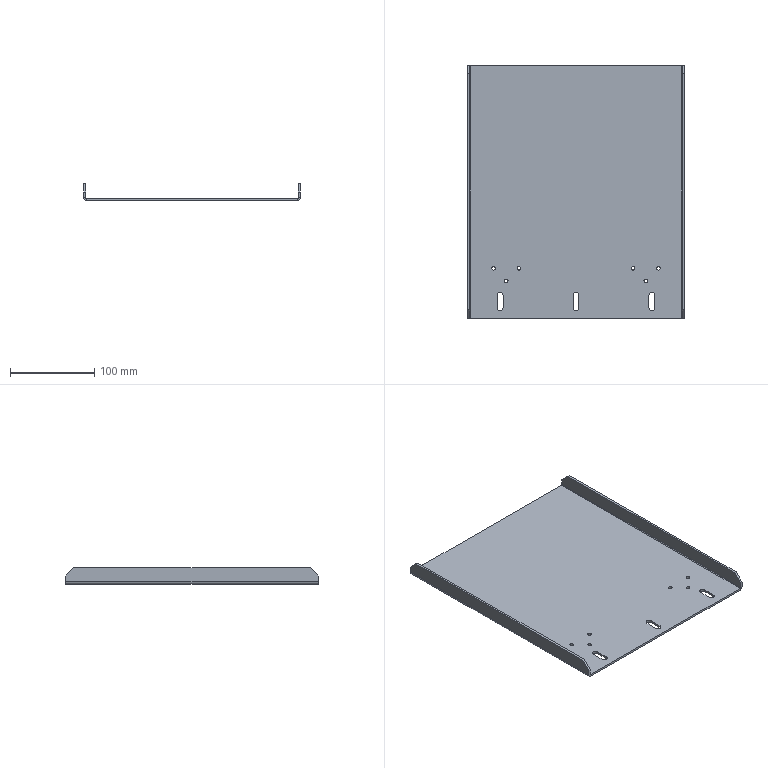Part | SolidWorks | features HoleWzd 2, BreakCorner 1, Chamfer 1, EdgeFlange 1, Extrusion 1, FlatPattern 1, SheetMetal 1, SolidToSheetMetal 1 | 1 solid | 50 faces | box 257 x 300 x 20 mm | volume 215937 mm3 | plane 28 | cylinder 22 | commonest cylinder face diameters 4.2 x12 7 x6 1.473 x2 6.473 x2
STEP:
#1=CARTESIAN_POINT('',(-95.65,-90.5,1.5));
#2=VERTEX_POINT('',#1);
#3=CARTESIAN_POINT('',(-99.85,-90.5,1.5));
#4=VERTEX_POINT('',#3);
#5=CARTESIAN_POINT('',(-97.75,-90.5,1.5));
#6=DIRECTION('',(0.,0.,-1.));
#7=DIRECTION('',(-1.,0.,0.));
#8=AXIS2_PLACEMENT_3D('',#5,#6,#7);
#9=CIRCLE('',#8,2.1);
#10=EDGE_CURVE('',#2,#4,#9,.T.);
#11=ORIENTED_EDGE('',*,*,#10,.F.);
#12=CARTESIAN_POINT('',(-95.65,-90.5,-1.));
#13=VERTEX_POINT('',#12);
#14=CARTESIAN_POINT('',(-95.65,-90.5,1.5));
#15=DIRECTION('',(0.,0.,-1.));
#16=VECTOR('',#15,1000.);
#17=LINE('',#14,#16);
#18=EDGE_CURVE('',#2,#13,#17,.T.);
#19=ORIENTED_EDGE('',*,*,#18,.T.);
#20=CARTESIAN_POINT('',(-99.85,-90.5,-1.));
#21=VERTEX_POINT('',#20);
#22=CARTESIAN_POINT('',(-97.75,-90.5,-1.));
#23=DIRECTION('',(0.,0.,-1.));
#24=DIRECTION('',(-1.,0.,0.));
#25=AXIS2_PLACEMENT_3D('',#22,#23,#24);
#26=CIRCLE('',#25,2.1);
#27=EDGE_CURVE('',#13,#21,#26,.T.);
#28=ORIENTED_EDGE('',*,*,#27,.T.);
#29=CARTESIAN_POINT('',(-99.85,-90.5,1.5));
#30=DIRECTION('',(0.,0.,-1.));
#31=VECTOR('',#30,1000.);
#32=LINE('',#29,#31);
#33=EDGE_CURVE('',#4,#21,#32,.T.);
#34=ORIENTED_EDGE('',*,*,#33,.F.);
#35=EDGE_LOOP('',(#11,#19,#28,#34));
#36=FACE_OUTER_BOUND('',#35,.T.);
#37=CARTESIAN_POINT('',(-97.75,-90.5,1.5));
#38=DIRECTION('',(0.,0.,-1.));
#39=DIRECTION('',(-1.,0.,0.));
#40=AXIS2_PLACEMENT_3D('',#37,#38,#39);
#41=CYLINDRICAL_SURFACE('',#40,2.1);
#42=ADVANCED_FACE('',(#36),#41,.F.);
#43=CARTESIAN_POINT('',(-65.65,-90.5,1.5));
#44=VERTEX_POINT('',#43);
#45=CARTESIAN_POINT('',(-69.85,-90.5,1.5));
#46=VERTEX_POINT('',#45);
#47=CARTESIAN_POINT('',(-67.75,-90.5,1.5));
#48=DIRECTION('',(0.,0.,-1.));
#49=DIRECTION('',(-1.,0.,0.));
#50=AXIS2_PLACEMENT_3D('',#47,#48,#49);
#51=CIRCLE('',#50,2.1);
#52=EDGE_CURVE('',#44,#46,#51,.T.);
#53=ORIENTED_EDGE('',*,*,#52,.F.);
#54=CARTESIAN_POINT('',(-65.65,-90.5,-1.));
#55=VERTEX_POINT('',#54);
#56=CARTESIAN_POINT('',(-65.65,-90.5,1.5));
#57=DIRECTION('',(0.,0.,-1.));
#58=VECTOR('',#57,1000.);
#59=LINE('',#56,#58);
#60=EDGE_CURVE('',#44,#55,#59,.T.);
#61=ORIENTED_EDGE('',*,*,#60,.T.);
#62=CARTESIAN_POINT('',(-69.85,-90.5,-1.));
#63=VERTEX_POINT('',#62);
#64=CARTESIAN_POINT('',(-67.75,-90.5,-1.));
#65=DIRECTION('',(0.,0.,-1.));
#66=DIRECTION('',(-1.,0.,0.));
#67=AXIS2_PLACEMENT_3D('',#64,#65,#66);
#68=CIRCLE('',#67,2.1);
#69=EDGE_CURVE('',#55,#63,#68,.T.);
#70=ORIENTED_EDGE('',*,*,#69,.T.);
#71=CARTESIAN_POINT('',(-69.85,-90.5,1.5));
#72=DIRECTION('',(0.,0.,-1.));
#73=VECTOR('',#72,1000.);
#74=LINE('',#71,#73);
#75=EDGE_CURVE('',#46,#63,#74,.T.);
#76=ORIENTED_EDGE('',*,*,#75,.F.);
#77=EDGE_LOOP('',(#53,#61,#70,#76));
#78=FACE_OUTER_BOUND('',#77,.T.);
#79=CARTESIAN_POINT('',(-67.75,-90.5,1.5));
#80=DIRECTION('',(0.,0.,-1.));
#81=DIRECTION('',(-1.,0.,0.));
#82=AXIS2_PLACEMENT_3D('',#79,#80,#81);
#83=CYLINDRICAL_SURFACE('',#82,2.1);
#84=ADVANCED_FACE('',(#78),#83,.F.);
#85=CARTESIAN_POINT('',(-80.65,-105.5,1.5));
#86=VERTEX_POINT('',#85);
#87=CARTESIAN_POINT('',(-84.85,-105.5,1.5));
#88=VERTEX_POINT('',#87);
#89=CARTESIAN_POINT('',(-82.75,-105.5,1.5));
#90=DIRECTION('',(0.,0.,-1.));
#91=DIRECTION('',(-1.,0.,0.));
#92=AXIS2_PLACEMENT_3D('',#89,#90,#91);
#93=CIRCLE('',#92,2.1);
#94=EDGE_CURVE('',#86,#88,#93,.T.);
#95=ORIENTED_EDGE('',*,*,#94,.F.);
#96=CARTESIAN_POINT('',(-80.65,-105.5,-1.));
#97=VERTEX_POINT('',#96);
#98=CARTESIAN_POINT('',(-80.65,-105.5,1.5));
#99=DIRECTION('',(0.,0.,-1.));
#100=VECTOR('',#99,1000.);
#101=LINE('',#98,#100);
#102=EDGE_CURVE('',#86,#97,#101,.T.);
#103=ORIENTED_EDGE('',*,*,#102,.T.);
#104=CARTESIAN_POINT('',(-84.85,-105.5,-1.));
#105=VERTEX_POINT('',#104);
#106=CARTESIAN_POINT('',(-82.75,-105.5,-1.));
#107=DIRECTION('',(0.,0.,-1.));
#108=DIRECTION('',(-1.,0.,0.));
#109=AXIS2_PLACEMENT_3D('',#106,#107,#108);
#110=CIRCLE('',#109,2.1);
#111=EDGE_CURVE('',#97,#105,#110,.T.);
#112=ORIENTED_EDGE('',*,*,#111,.T.);
#113=CARTESIAN_POINT('',(-84.85,-105.5,1.5));
#114=DIRECTION('',(0.,0.,-1.));
#115=VECTOR('',#114,1000.);
#116=LINE('',#113,#115);
#117=EDGE_CURVE('',#88,#105,#116,.T.);
#118=ORIENTED_EDGE('',*,*,#117,.F.);
#119=EDGE_LOOP('',(#95,#103,#112,#118));
#120=FACE_OUTER_BOUND('',#119,.T.);
#121=CARTESIAN_POINT('',(-82.75,-105.5,1.5));
#122=DIRECTION('',(0.,0.,-1.));
#123=DIRECTION('',(-1.,0.,0.));
#124=AXIS2_PLACEMENT_3D('',#121,#122,#123);
#125=CYLINDRICAL_SURFACE('',#124,2.1);
#126=ADVANCED_FACE('',(#120),#125,.F.);
#127=CARTESIAN_POINT('',(84.85,-105.5,1.5));
#128=VERTEX_POINT('',#127);
#129=CARTESIAN_POINT('',(80.65,-105.5,1.5));
#130=VERTEX_POINT('',#129);
#131=CARTESIAN_POINT('',(82.75,-105.5,1.5));
#132=DIRECTION('',(0.,0.,-1.));
#133=DIRECTION('',(-1.,0.,0.));
#134=AXIS2_PLACEMENT_3D('',#131,#132,#133);
#135=CIRCLE('',#134,2.1);
#136=EDGE_CURVE('',#128,#130,#135,.T.);
#137=ORIENTED_EDGE('',*,*,#136,.F.);
#138=CARTESIAN_POINT('',(84.85,-105.5,-1.));
#139=VERTEX_POINT('',#138);
#140=CARTESIAN_POINT('',(84.85,-105.5,1.5));
#141=DIRECTION('',(0.,0.,-1.));
#142=VECTOR('',#141,1000.);
#143=LINE('',#140,#142);
#144=EDGE_CURVE('',#128,#139,#143,.T.);
#145=ORIENTED_EDGE('',*,*,#144,.T.);
#146=CARTESIAN_POINT('',(80.65,-105.5,-1.));
#147=VERTEX_POINT('',#146);
#148=CARTESIAN_POINT('',(82.75,-105.5,-1.));
#149=DIRECTION('',(0.,0.,-1.));
#150=DIRECTION('',(-1.,0.,0.));
#151=AXIS2_PLACEMENT_3D('',#148,#149,#150);
#152=CIRCLE('',#151,2.1);
#153=EDGE_CURVE('',#139,#147,#152,.T.);
#154=ORIENTED_EDGE('',*,*,#153,.T.);
#155=CARTESIAN_POINT('',(80.65,-105.5,1.5));
#156=DIRECTION('',(0.,0.,-1.));
#157=VECTOR('',#156,1000.);
#158=LINE('',#155,#157);
#159=EDGE_CURVE('',#130,#147,#158,.T.);
#160=ORIENTED_EDGE('',*,*,#159,.F.);
#161=EDGE_LOOP('',(#137,#145,#154,#160));
#162=FACE_OUTER_BOUND('',#161,.T.);
#163=CARTESIAN_POINT('',(82.75,-105.5,1.5));
#164=DIRECTION('',(0.,0.,-1.));
#165=DIRECTION('',(-1.,0.,0.));
#166=AXIS2_PLACEMENT_3D('',#163,#164,#165);
#167=CYLINDRICAL_SURFACE('',#166,2.1);
#168=ADVANCED_FACE('',(#162),#167,.F.);
#169=CARTESIAN_POINT('',(69.85,-90.5,1.5));
#170=VERTEX_POINT('',#169);
#171=CARTESIAN_POINT('',(65.65,-90.5,1.5));
#172=VERTEX_POINT('',#171);
#173=CARTESIAN_POINT('',(67.75,-90.5,1.5));
#174=DIRECTION('',(0.,0.,-1.));
#175=DIRECTION('',(-1.,0.,0.));
#176=AXIS2_PLACEMENT_3D('',#173,#174,#175);
#177=CIRCLE('',#176,2.1);
#178=EDGE_CURVE('',#170,#172,#177,.T.);
#179=ORIENTED_EDGE('',*,*,#178,.F.);
#180=CARTESIAN_POINT('',(69.85,-90.5,-1.));
#181=VERTEX_POINT('',#180);
#182=CARTESIAN_POINT('',(69.85,-90.5,1.5));
#183=DIRECTION('',(0.,0.,-1.));
#184=VECTOR('',#183,1000.);
#185=LINE('',#182,#184);
#186=EDGE_CURVE('',#170,#181,#185,.T.);
#187=ORIENTED_EDGE('',*,*,#186,.T.);
#188=CARTESIAN_POINT('',(65.65,-90.5,-1.));
#189=VERTEX_POINT('',#188);
#190=CARTESIAN_POINT('',(67.75,-90.5,-1.));
#191=DIRECTION('',(0.,0.,-1.));
#192=DIRECTION('',(-1.,0.,0.));
#193=AXIS2_PLACEMENT_3D('',#190,#191,#192);
#194=CIRCLE('',#193,2.1);
#195=EDGE_CURVE('',#181,#189,#194,.T.);
#196=ORIENTED_EDGE('',*,*,#195,.T.);
#197=CARTESIAN_POINT('',(65.65,-90.5,1.5));
#198=DIRECTION('',(0.,0.,-1.));
#199=VECTOR('',#198,1000.);
#200=LINE('',#197,#199);
#201=EDGE_CURVE('',#172,#189,#200,.T.);
#202=ORIENTED_EDGE('',*,*,#201,.F.);
#203=EDGE_LOOP('',(#179,#187,#196,#202));
#204=FACE_OUTER_BOUND('',#203,.T.);
#205=CARTESIAN_POINT('',(67.75,-90.5,1.5));
#206=DIRECTION('',(0.,0.,-1.));
#207=DIRECTION('',(-1.,0.,0.));
#208=AXIS2_PLACEMENT_3D('',#205,#206,#207);
#209=CYLINDRICAL_SURFACE('',#208,2.1);
#210=ADVANCED_FACE('',(#204),#209,.F.);
#211=CARTESIAN_POINT('',(99.85,-90.5,1.5));
#212=VERTEX_POINT('',#211);
#213=CARTESIAN_POINT('',(95.65,-90.5,1.5));
#214=VERTEX_POINT('',#213);
#215=CARTESIAN_POINT('',(97.75,-90.5,1.5));
#216=DIRECTION('',(0.,0.,-1.));
#217=DIRECTION('',(-1.,0.,0.));
#218=AXIS2_PLACEMENT_3D('',#215,#216,#217);
#219=CIRCLE('',#218,2.1);
#220=EDGE_CURVE('',#212,#214,#219,.T.);
#221=ORIENTED_EDGE('',*,*,#220,.F.);
#222=CARTESIAN_POINT('',(99.85,-90.5,-1.));
#223=VERTEX_POINT('',#222);
#224=CARTESIAN_POINT('',(99.85,-90.5,1.5));
#225=DIRECTION('',(0.,0.,-1.));
#226=VECTOR('',#225,1000.);
#227=LINE('',#224,#226);
#228=EDGE_CURVE('',#212,#223,#227,.T.);
#229=ORIENTED_EDGE('',*,*,#228,.T.);
#230=CARTESIAN_POINT('',(95.65,-90.5,-1.));
#231=VERTEX_POINT('',#230);
#232=CARTESIAN_POINT('',(97.75,-90.5,-1.));
#233=DIRECTION('',(0.,0.,-1.));
#234=DIRECTION('',(-1.,0.,0.));
#235=AXIS2_PLACEMENT_3D('',#232,#233,#234);
#236=CIRCLE('',#235,2.1);
#237=EDGE_CURVE('',#223,#231,#236,.T.);
#238=ORIENTED_EDGE('',*,*,#237,.T.);
#239=CARTESIAN_POINT('',(95.65,-90.5,1.5));
#240=DIRECTION('',(0.,0.,-1.));
#241=VECTOR('',#240,1000.);
#242=LINE('',#239,#241);
#243=EDGE_CURVE('',#214,#231,#242,.T.);
#244=ORIENTED_EDGE('',*,*,#243,.F.);
#245=EDGE_LOOP('',(#221,#229,#238,#244));
#246=FACE_OUTER_BOUND('',#245,.T.);
#247=CARTESIAN_POINT('',(97.75,-90.5,1.5));
#248=DIRECTION('',(0.,0.,-1.));
#249=DIRECTION('',(-1.,0.,0.));
#250=AXIS2_PLACEMENT_3D('',#247,#248,#249);
#251=CYLINDRICAL_SURFACE('',#250,2.1);
#252=ADVANCED_FACE('',(#246),#251,.F.);
#253=CARTESIAN_POINT('',(97.75,-90.5,1.5));
#254=DIRECTION('',(0.,0.,-1.));
#255=DIRECTION('',(-1.,0.,0.));
#256=AXIS2_PLACEMENT_3D('',#253,#254,#255);
#257=CIRCLE('',#256,2.1);
#258=EDGE_CURVE('',#214,#212,#257,.T.);
#259=ORIENTED_EDGE('',*,*,#258,.T.);
#260=ORIENTED_EDGE('',*,*,#220,.T.);
#261=EDGE_LOOP('',(#259,#260));
#262=FACE_BOUND('',#261,.T.);
#263=CARTESIAN_POINT('',(67.75,-90.5,1.5));
#264=DIRECTION('',(0.,0.,-1.));
#265=DIRECTION('',(-1.,0.,0.));
#266=AXIS2_PLACEMENT_3D('',#263,#264,#265);
#267=CIRCLE('',#266,2.1);
#268=EDGE_CURVE('',#172,#170,#267,.T.);
#269=ORIENTED_EDGE('',*,*,#268,.T.);
#270=ORIENTED_EDGE('',*,*,#178,.T.);
#271=EDGE_LOOP('',(#269,#270));
#272=FACE_BOUND('',#271,.T.);
#273=CARTESIAN_POINT('',(82.75,-105.5,1.5));
#274=DIRECTION('',(0.,0.,-1.));
#275=DIRECTION('',(-1.,0.,0.));
#276=AXIS2_PLACEMENT_3D('',#273,#274,#275);
#277=CIRCLE('',#276,2.1);
#278=EDGE_CURVE('',#130,#128,#277,.T.);
#279=ORIENTED_EDGE('',*,*,#278,.T.);
#280=ORIENTED_EDGE('',*,*,#136,.T.);
#281=EDGE_LOOP('',(#279,#280));
#282=FACE_BOUND('',#281,.T.);
#283=CARTESIAN_POINT('',(-82.75,-105.5,1.5));
#284=DIRECTION('',(0.,0.,-1.));
#285=DIRECTION('',(-1.,0.,0.));
#286=AXIS2_PLACEMENT_3D('',#283,#284,#285);
#287=CIRCLE('',#286,2.1);
#288=EDGE_CURVE('',#88,#86,#287,.T.);
#289=ORIENTED_EDGE('',*,*,#288,.T.);
#290=ORIENTED_EDGE('',*,*,#94,.T.);
#291=EDGE_LOOP('',(#289,#290));
#292=FACE_BOUND('',#291,.T.);
#293=CARTESIAN_POINT('',(-67.75,-90.5,1.5));
#294=DIRECTION('',(0.,0.,-1.));
#295=DIRECTION('',(-1.,0.,0.));
#296=AXIS2_PLACEMENT_3D('',#293,#294,#295);
#297=CIRCLE('',#296,2.1);
#298=EDGE_CURVE('',#46,#44,#297,.T.);
#299=ORIENTED_EDGE('',*,*,#298,.T.);
#300=ORIENTED_EDGE('',*,*,#52,.T.);
#301=EDGE_LOOP('',(#299,#300));
#302=FACE_BOUND('',#301,.T.);
#303=CARTESIAN_POINT('',(-97.75,-90.5,1.5));
#304=DIRECTION('',(0.,0.,-1.));
#305=DIRECTION('',(-1.,0.,0.));
#306=AXIS2_PLACEMENT_3D('',#303,#304,#305);
#307=CIRCLE('',#306,2.1);
#308=EDGE_CURVE('',#4,#2,#307,.T.);
#309=ORIENTED_EDGE('',*,*,#308,.T.);
#310=ORIENTED_EDGE('',*,*,#10,.T.);
#311=EDGE_LOOP('',(#309,#310));
#312=FACE_BOUND('',#311,.T.);
#313=CARTESIAN_POINT('',(93.5,-137.5,1.5));
#314=VERTEX_POINT('',#313);
#315=CARTESIAN_POINT('',(93.5,-122.5,1.5));
#316=VERTEX_POINT('',#315);
#317=CARTESIAN_POINT('',(93.5,-137.5,1.5));
#318=DIRECTION('',(0.,1.,0.));
#319=VECTOR('',#318,1000.);
#320=LINE('',#317,#319);
#321=EDGE_CURVE('',#314,#316,#320,.T.);
#322=ORIENTED_EDGE('',*,*,#321,.F.);
#323=CARTESIAN_POINT('',(86.5,-137.5,1.5));
#324=VERTEX_POINT('',#323);
#325=CARTESIAN_POINT('',(90.,-137.5,1.5));
#326=DIRECTION('',(0.,0.,-1.));
#327=DIRECTION('',(-1.,0.,0.));
#328=AXIS2_PLACEMENT_3D('',#325,#326,#327);
#329=CIRCLE('',#328,3.5);
#330=EDGE_CURVE('',#314,#324,#329,.T.);
#331=ORIENTED_EDGE('',*,*,#330,.T.);
#332=CARTESIAN_POINT('',(86.5,-122.5,1.5));
#333=VERTEX_POINT('',#332);
#334=CARTESIAN_POINT('',(86.5,-137.5,1.5));
#335=DIRECTION('',(0.,1.,0.));
#336=VECTOR('',#335,1000.);
#337=LINE('',#334,#336);
#338=EDGE_CURVE('',#324,#333,#337,.T.);
#339=ORIENTED_EDGE('',*,*,#338,.T.);
#340=CARTESIAN_POINT('',(90.,-122.5,1.5));
#341=DIRECTION('',(0.,0.,-1.));
#342=DIRECTION('',(-1.,0.,0.));
#343=AXIS2_PLACEMENT_3D('',#340,#341,#342);
#344=CIRCLE('',#343,3.5);
#345=EDGE_CURVE('',#333,#316,#344,.T.);
#346=ORIENTED_EDGE('',*,*,#345,.T.);
#347=EDGE_LOOP('',(#322,#331,#339,#346));
#348=FACE_BOUND('',#347,.T.);
#349=CARTESIAN_POINT('',(-93.5,-137.5,1.5));
#350=VERTEX_POINT('',#349);
#351=CARTESIAN_POINT('',(-93.5,-122.5,1.5));
#352=VERTEX_POINT('',#351);
#353=CARTESIAN_POINT('',(-93.5,-137.5,1.5));
#354=DIRECTION('',(0.,1.,0.));
#355=VECTOR('',#354,1000.);
#356=LINE('',#353,#355);
#357=EDGE_CURVE('',#350,#352,#356,.T.);
#358=ORIENTED_EDGE('',*,*,#357,.T.);
#359=CARTESIAN_POINT('',(-86.5,-122.5,1.5));
#360=VERTEX_POINT('',#359);
#361=CARTESIAN_POINT('',(-90.,-122.5,1.5));
#362=DIRECTION('',(0.,0.,-1.));
#363=DIRECTION('',(-1.,0.,0.));
#364=AXIS2_PLACEMENT_3D('',#361,#362,#363);
#365=CIRCLE('',#364,3.5);
#366=EDGE_CURVE('',#352,#360,#365,.T.);
#367=ORIENTED_EDGE('',*,*,#366,.T.);
#368=CARTESIAN_POINT('',(-86.5,-137.5,1.5));
#369=VERTEX_POINT('',#368);
#370=CARTESIAN_POINT('',(-86.5,-137.5,1.5));
#371=DIRECTION('',(0.,1.,0.));
#372=VECTOR('',#371,1000.);
#373=LINE('',#370,#372);
#374=EDGE_CURVE('',#369,#360,#373,.T.);
#375=ORIENTED_EDGE('',*,*,#374,.F.);
#376=CARTESIAN_POINT('',(-90.,-137.5,1.5));
#377=DIRECTION('',(0.,0.,-1.));
#378=DIRECTION('',(-1.,0.,0.));
#379=AXIS2_PLACEMENT_3D('',#376,#377,#378);
#380=CIRCLE('',#379,3.5);
#381=EDGE_CURVE('',#369,#350,#380,.T.);
#382=ORIENTED_EDGE('',*,*,#381,.T.);
#383=EDGE_LOOP('',(#358,#367,#375,#382));
#384=FACE_BOUND('',#383,.T.);
#385=CARTESIAN_POINT('',(3.5,-137.5,1.5));
#386=VERTEX_POINT('',#385);
#387=CARTESIAN_POINT('',(3.5,-122.5,1.5));
#388=VERTEX_POINT('',#387);
#389=CARTESIAN_POINT('',(3.5,-137.5,1.5));
#390=DIRECTION('',(0.,1.,0.));
#391=VECTOR('',#390,1000.);
#392=LINE('',#389,#391);
#393=EDGE_CURVE('',#386,#388,#392,.T.);
#394=ORIENTED_EDGE('',*,*,#393,.F.);
#395=CARTESIAN_POINT('',(-3.5,-137.5,1.5));
#396=VERTEX_POINT('',#395);
#397=CARTESIAN_POINT('',(0.,-137.5,1.5));
#398=DIRECTION('',(0.,0.,-1.));
#399=DIRECTION('',(-1.,0.,0.));
#400=AXIS2_PLACEMENT_3D('',#397,#398,#399);
#401=CIRCLE('',#400,3.5);
#402=EDGE_CURVE('',#386,#396,#401,.T.);
#403=ORIENTED_EDGE('',*,*,#402,.T.);
#404=CARTESIAN_POINT('',(-3.5,-122.5,1.5));
#405=VERTEX_POINT('',#404);
#406=CARTESIAN_POINT('',(-3.5,-137.5,1.5));
#407=DIRECTION('',(0.,1.,0.));
#408=VECTOR('',#407,1000.);
#409=LINE('',#406,#408);
#410=EDGE_CURVE('',#396,#405,#409,.T.);
#411=ORIENTED_EDGE('',*,*,#410,.T.);
#412=CARTESIAN_POINT('',(0.,-122.5,1.5));
#413=DIRECTION('',(0.,0.,-1.));
#414=DIRECTION('',(-1.,0.,0.));
#415=AXIS2_PLACEMENT_3D('',#412,#413,#414);
#416=CIRCLE('',#415,3.5);
#417=EDGE_CURVE('',#405,#388,#416,.T.);
#418=ORIENTED_EDGE('',*,*,#417,.T.);
#419=EDGE_LOOP('',(#394,#403,#411,#418));
#420=FACE_BOUND('',#419,.T.);
#421=CARTESIAN_POINT('',(-125.263,-150.,1.5));
#422=VERTEX_POINT('',#421);
#423=CARTESIAN_POINT('',(-125.263,150.,1.5));
#424=VERTEX_POINT('',#423);
#425=CARTESIAN_POINT('',(-125.263,-150.,1.5));
#426=DIRECTION('',(0.,1.,0.));
#427=VECTOR('',#426,1000.);
#428=LINE('',#425,#427);
#429=EDGE_CURVE('',#422,#424,#428,.T.);
#430=ORIENTED_EDGE('',*,*,#429,.F.);
#431=CARTESIAN_POINT('',(125.263,-150.,1.5));
#432=VERTEX_POINT('',#431);
#433=CARTESIAN_POINT('',(-126.,-150.,1.5));
#434=DIRECTION('',(1.,0.,0.));
#435=VECTOR('',#434,1000.);
#436=LINE('',#433,#435);
#437=EDGE_CURVE('',#422,#432,#436,.T.);
#438=ORIENTED_EDGE('',*,*,#437,.T.);
#439=CARTESIAN_POINT('',(125.263,150.,1.5));
#440=VERTEX_POINT('',#439);
#441=CARTESIAN_POINT('',(125.263,150.,1.5));
#442=DIRECTION('',(0.,-1.,0.));
#443=VECTOR('',#442,1000.);
#444=LINE('',#441,#443);
#445=EDGE_CURVE('',#440,#432,#444,.T.);
#446=ORIENTED_EDGE('',*,*,#445,.F.);
#447=CARTESIAN_POINT('',(-126.,150.,1.5));
#448=DIRECTION('',(-1.,0.,0.));
#449=VECTOR('',#448,1000.);
#450=LINE('',#447,#449);
#451=EDGE_CURVE('',#440,#424,#450,.T.);
#452=ORIENTED_EDGE('',*,*,#451,.T.);
#453=EDGE_LOOP('',(#430,#438,#446,#452));
#454=FACE_OUTER_BOUND('',#453,.T.);
#455=CARTESIAN_POINT('',(0.,0.,1.5));
#456=DIRECTION('',(0.,0.,-1.));
#457=DIRECTION('',(-1.,0.,0.));
#458=AXIS2_PLACEMENT_3D('',#455,#456,#457);
#459=PLANE('',#458);
#460=ADVANCED_FACE('',(#262,#272,#282,#292,#302,#312,#348,#384,#420,#454),#459,.F.);
#461=CARTESIAN_POINT('',(97.75,-90.5,-1.));
#462=DIRECTION('',(0.,0.,-1.));
#463=DIRECTION('',(-1.,0.,0.));
#464=AXIS2_PLACEMENT_3D('',#461,#462,#463);
#465=CIRCLE('',#464,2.1);
#466=EDGE_CURVE('',#231,#223,#465,.T.);
#467=ORIENTED_EDGE('',*,*,#466,.F.);
#468=ORIENTED_EDGE('',*,*,#237,.F.);
#469=EDGE_LOOP('',(#467,#468));
#470=FACE_BOUND('',#469,.T.);
#471=CARTESIAN_POINT('',(67.75,-90.5,-1.));
#472=DIRECTION('',(0.,0.,-1.));
#473=DIRECTION('',(-1.,0.,0.));
#474=AXIS2_PLACEMENT_3D('',#471,#472,#473);
#475=CIRCLE('',#474,2.1);
#476=EDGE_CURVE('',#189,#181,#475,.T.);
#477=ORIENTED_EDGE('',*,*,#476,.F.);
#478=ORIENTED_EDGE('',*,*,#195,.F.);
#479=EDGE_LOOP('',(#477,#478));
#480=FACE_BOUND('',#479,.T.);
#481=CARTESIAN_POINT('',(82.75,-105.5,-1.));
#482=DIRECTION('',(0.,0.,-1.));
#483=DIRECTION('',(-1.,0.,0.));
#484=AXIS2_PLACEMENT_3D('',#481,#482,#483);
#485=CIRCLE('',#484,2.1);
#486=EDGE_CURVE('',#147,#139,#485,.T.);
#487=ORIENTED_EDGE('',*,*,#486,.F.);
#488=ORIENTED_EDGE('',*,*,#153,.F.);
#489=EDGE_LOOP('',(#487,#488));
#490=FACE_BOUND('',#489,.T.);
#491=CARTESIAN_POINT('',(-82.75,-105.5,-1.));
#492=DIRECTION('',(0.,0.,-1.));
#493=DIRECTION('',(-1.,0.,0.));
#494=AXIS2_PLACEMENT_3D('',#491,#492,#493);
#495=CIRCLE('',#494,2.1);
#496=EDGE_CURVE('',#105,#97,#495,.T.);
#497=ORIENTED_EDGE('',*,*,#496,.F.);
#498=ORIENTED_EDGE('',*,*,#111,.F.);
#499=EDGE_LOOP('',(#497,#498));
#500=FACE_BOUND('',#499,.T.);
#501=CARTESIAN_POINT('',(-67.75,-90.5,-1.));
#502=DIRECTION('',(0.,0.,-1.));
#503=DIRECTION('',(-1.,0.,0.));
#504=AXIS2_PLACEMENT_3D('',#501,#502,#503);
#505=CIRCLE('',#504,2.1);
#506=EDGE_CURVE('',#63,#55,#505,.T.);
#507=ORIENTED_EDGE('',*,*,#506,.F.);
#508=ORIENTED_EDGE('',*,*,#69,.F.);
#509=EDGE_LOOP('',(#507,#508));
#510=FACE_BOUND('',#509,.T.);
#511=CARTESIAN_POINT('',(-97.75,-90.5,-1.));
#512=DIRECTION('',(0.,0.,-1.));
#513=DIRECTION('',(-1.,0.,0.));
#514=AXIS2_PLACEMENT_3D('',#511,#512,#513);
#515=CIRCLE('',#514,2.1);
#516=EDGE_CURVE('',#21,#13,#515,.T.);
#517=ORIENTED_EDGE('',*,*,#516,.F.);
#518=ORIENTED_EDGE('',*,*,#27,.F.);
#519=EDGE_LOOP('',(#517,#518));
#520=FACE_BOUND('',#519,.T.);
#521=CARTESIAN_POINT('',(93.5,-137.5,-1.));
#522=VERTEX_POINT('',#521);
#523=CARTESIAN_POINT('',(93.5,-122.5,-1.));
#524=VERTEX_POINT('',#523);
#525=CARTESIAN_POINT('',(93.5,0.,-1.));
#526=DIRECTION('',(0.,1.,0.));
#527=VECTOR('',#526,1000.);
#528=LINE('',#525,#527);
#529=EDGE_CURVE('',#522,#524,#528,.T.);
#530=ORIENTED_EDGE('',*,*,#529,.T.);
#531=CARTESIAN_POINT('',(86.5,-122.5,-1.));
#532=VERTEX_POINT('',#531);
#533=CARTESIAN_POINT('',(90.,-122.5,-1.));
#534=DIRECTION('',(0.,0.,-1.));
#535=DIRECTION('',(-1.,0.,0.));
#536=AXIS2_PLACEMENT_3D('',#533,#534,#535);
#537=CIRCLE('',#536,3.5);
#538=EDGE_CURVE('',#532,#524,#537,.T.);
#539=ORIENTED_EDGE('',*,*,#538,.F.);
#540=CARTESIAN_POINT('',(86.5,-137.5,-1.));
#541=VERTEX_POINT('',#540);
#542=CARTESIAN_POINT('',(86.5,0.,-1.));
#543=DIRECTION('',(0.,1.,0.));
#544=VECTOR('',#543,1000.);
#545=LINE('',#542,#544);
#546=EDGE_CURVE('',#541,#532,#545,.T.);
#547=ORIENTED_EDGE('',*,*,#546,.F.);
#548=CARTESIAN_POINT('',(90.,-137.5,-1.));
#549=DIRECTION('',(0.,0.,-1.));
#550=DIRECTION('',(-1.,0.,0.));
#551=AXIS2_PLACEMENT_3D('',#548,#549,#550);
#552=CIRCLE('',#551,3.5);
#553=EDGE_CURVE('',#522,#541,#552,.T.);
#554=ORIENTED_EDGE('',*,*,#553,.F.);
#555=EDGE_LOOP('',(#530,#539,#547,#554));
#556=FACE_BOUND('',#555,.T.);
#557=CARTESIAN_POINT('',(-93.5,-137.5,-1.));
#558=VERTEX_POINT('',#557);
#559=CARTESIAN_POINT('',(-93.5,-122.5,-1.));
#560=VERTEX_POINT('',#559);
#561=CARTESIAN_POINT('',(-93.5,0.,-1.));
#562=DIRECTION('',(0.,1.,0.));
#563=VECTOR('',#562,1000.);
#564=LINE('',#561,#563);
#565=EDGE_CURVE('',#558,#560,#564,.T.);
#566=ORIENTED_EDGE('',*,*,#565,.F.);
#567=CARTESIAN_POINT('',(-86.5,-137.5,-1.));
#568=VERTEX_POINT('',#567);
#569=CARTESIAN_POINT('',(-90.,-137.5,-1.));
#570=DIRECTION('',(0.,0.,-1.));
#571=DIRECTION('',(-1.,0.,0.));
#572=AXIS2_PLACEMENT_3D('',#569,#570,#571);
#573=CIRCLE('',#572,3.5);
#574=EDGE_CURVE('',#568,#558,#573,.T.);
#575=ORIENTED_EDGE('',*,*,#574,.F.);
#576=CARTESIAN_POINT('',(-86.5,-122.5,-1.));
#577=VERTEX_POINT('',#576);
#578=CARTESIAN_POINT('',(-86.5,0.,-1.));
#579=DIRECTION('',(0.,1.,0.));
#580=VECTOR('',#579,1000.);
#581=LINE('',#578,#580);
#582=EDGE_CURVE('',#568,#577,#581,.T.);
#583=ORIENTED_EDGE('',*,*,#582,.T.);
#584=CARTESIAN_POINT('',(-90.,-122.5,-1.));
#585=DIRECTION('',(0.,0.,-1.));
#586=DIRECTION('',(-1.,0.,0.));
#587=AXIS2_PLACEMENT_3D('',#584,#585,#586);
#588=CIRCLE('',#587,3.5);
#589=EDGE_CURVE('',#560,#577,#588,.T.);
#590=ORIENTED_EDGE('',*,*,#589,.F.);
#591=EDGE_LOOP('',(#566,#575,#583,#590));
#592=FACE_BOUND('',#591,.T.);
#593=CARTESIAN_POINT('',(3.5,-137.5,-1.));
#594=VERTEX_POINT('',#593);
#595=CARTESIAN_POINT('',(3.5,-122.5,-1.));
#596=VERTEX_POINT('',#595);
#597=CARTESIAN_POINT('',(3.5,0.,-1.));
#598=DIRECTION('',(0.,1.,0.));
#599=VECTOR('',#598,1000.);
#600=LINE('',#597,#599);
#601=EDGE_CURVE('',#594,#596,#600,.T.);
#602=ORIENTED_EDGE('',*,*,#601,.T.);
#603=CARTESIAN_POINT('',(-3.5,-122.5,-1.));
#604=VERTEX_POINT('',#603);
#605=CARTESIAN_POINT('',(0.,-122.5,-1.));
#606=DIRECTION('',(0.,0.,-1.));
#607=DIRECTION('',(-1.,0.,0.));
#608=AXIS2_PLACEMENT_3D('',#605,#606,#607);
#609=CIRCLE('',#608,3.5);
#610=EDGE_CURVE('',#604,#596,#609,.T.);
#611=ORIENTED_EDGE('',*,*,#610,.F.);
#612=CARTESIAN_POINT('',(-3.5,-137.5,-1.));
#613=VERTEX_POINT('',#612);
#614=CARTESIAN_POINT('',(-3.5,0.,-1.));
#615=DIRECTION('',(0.,1.,0.));
#616=VECTOR('',#615,1000.);
#617=LINE('',#614,#616);
#618=EDGE_CURVE('',#613,#604,#617,.T.);
#619=ORIENTED_EDGE('',*,*,#618,.F.);
#620=CARTESIAN_POINT('',(0.,-137.5,-1.));
#621=DIRECTION('',(0.,0.,-1.));
#622=DIRECTION('',(-1.,0.,0.));
#623=AXIS2_PLACEMENT_3D('',#620,#621,#622);
#624=CIRCLE('',#623,3.5);
#625=EDGE_CURVE('',#594,#613,#624,.T.);
#626=ORIENTED_EDGE('',*,*,#625,.F.);
#627=EDGE_LOOP('',(#602,#611,#619,#626));
#628=FACE_BOUND('',#627,.T.);
#629=CARTESIAN_POINT('',(-125.263,-150.,-1.));
#630=VERTEX_POINT('',#629);
#631=CARTESIAN_POINT('',(125.263,-150.,-1.));
#632=VERTEX_POINT('',#631);
#633=CARTESIAN_POINT('',(0.,-150.,-1.));
#634=DIRECTION('',(1.,0.,0.));
#635=VECTOR('',#634,1000.);
#636=LINE('',#633,#635);
#637=EDGE_CURVE('',#630,#632,#636,.T.);
#638=ORIENTED_EDGE('',*,*,#637,.F.);
#639=CARTESIAN_POINT('',(-125.263,150.,-1.));
#640=VERTEX_POINT('',#639);
#641=CARTESIAN_POINT('',(-125.263,-150.,-1.));
#642=DIRECTION('',(0.,1.,0.));
#643=VECTOR('',#642,1000.);
#644=LINE('',#641,#643);
#645=EDGE_CURVE('',#630,#640,#644,.T.);
#646=ORIENTED_EDGE('',*,*,#645,.T.);
#647=CARTESIAN_POINT('',(125.263,150.,-1.));
#648=VERTEX_POINT('',#647);
#649=CARTESIAN_POINT('',(0.,150.,-1.));
#650=DIRECTION('',(-1.,0.,0.));
#651=VECTOR('',#650,1000.);
#652=LINE('',#649,#651);
#653=EDGE_CURVE('',#648,#640,#652,.T.);
#654=ORIENTED_EDGE('',*,*,#653,.F.);
#655=CARTESIAN_POINT('',(125.263,150.,-1.));
#656=DIRECTION('',(0.,-1.,0.));
#657=VECTOR('',#656,1000.);
#658=LINE('',#655,#657);
#659=EDGE_CURVE('',#648,#632,#658,.T.);
#660=ORIENTED_EDGE('',*,*,#659,.T.);
#661=EDGE_LOOP('',(#638,#646,#654,#660));
#662=FACE_OUTER_BOUND('',#661,.T.);
#663=CARTESIAN_POINT('',(0.,0.,-1.));
#664=DIRECTION('',(0.,0.,-1.));
#665=DIRECTION('',(-1.,0.,0.));
#666=AXIS2_PLACEMENT_3D('',#663,#664,#665);
#667=PLANE('',#666);
#668=ADVANCED_FACE('',(#470,#480,#490,#500,#510,#520,#556,#592,#628,#662),#667,.T.);
#669=ORIENTED_EDGE('',*,*,#437,.F.);
#670=CARTESIAN_POINT('',(-125.263,-150.,1.5));
#671=DIRECTION('',(0.,0.,-1.));
#672=VECTOR('',#671,1000.);
#673=LINE('',#670,#672);
#674=EDGE_CURVE('',#422,#630,#673,.T.);
#675=ORIENTED_EDGE('',*,*,#674,.T.);
#676=ORIENTED_EDGE('',*,*,#637,.T.);
#677=CARTESIAN_POINT('',(125.263,-150.,1.5));
#678=DIRECTION('',(0.,0.,-1.));
#679=VECTOR('',#678,1000.);
#680=LINE('',#677,#679);
#681=EDGE_CURVE('',#432,#632,#680,.T.);
#682=ORIENTED_EDGE('',*,*,#681,.F.);
#683=EDGE_LOOP('',(#669,#675,#676,#682));
#684=FACE_OUTER_BOUND('',#683,.T.);
#685=CARTESIAN_POINT('',(-126.,-150.,1.5));
#686=DIRECTION('',(0.,1.,0.));
#687=DIRECTION('',(1.,0.,0.));
#688=AXIS2_PLACEMENT_3D('',#685,#686,#687);
#689=PLANE('',#688);
#690=ADVANCED_FACE('',(#684),#689,.F.);
#691=CARTESIAN_POINT('',(-125.263,150.,1.5));
#692=DIRECTION('',(0.,0.,-1.));
#693=VECTOR('',#692,1000.);
#694=LINE('',#691,#693);
#695=EDGE_CURVE('',#424,#640,#694,.T.);
#696=ORIENTED_EDGE('',*,*,#695,.F.);
#697=ORIENTED_EDGE('',*,*,#451,.F.);
#698=CARTESIAN_POINT('',(125.263,150.,1.5));
#699=DIRECTION('',(0.,0.,-1.));
#700=VECTOR('',#699,1000.);
#701=LINE('',#698,#700);
#702=EDGE_CURVE('',#440,#648,#701,.T.);
#703=ORIENTED_EDGE('',*,*,#702,.T.);
#704=ORIENTED_EDGE('',*,*,#653,.T.);
#705=EDGE_LOOP('',(#696,#697,#703,#704));
#706=FACE_OUTER_BOUND('',#705,.T.);
#707=CARTESIAN_POINT('',(-126.,150.,1.5));
#708=DIRECTION('',(0.,-1.,0.));
#709=DIRECTION('',(-1.,0.,0.));
#710=AXIS2_PLACEMENT_3D('',#707,#708,#709);
#711=PLANE('',#710);
#712=ADVANCED_FACE('',(#706),#711,.F.);
#713=CARTESIAN_POINT('',(-3.5,-137.5,1.5));
#714=DIRECTION('',(0.,0.,1.));
#715=VECTOR('',#714,1000.);
#716=LINE('',#713,#715);
#717=EDGE_CURVE('',#613,#396,#716,.T.);
#718=ORIENTED_EDGE('',*,*,#717,.F.);
#719=ORIENTED_EDGE('',*,*,#618,.T.);
#720=CARTESIAN_POINT('',(-3.5,-122.5,1.5));
#721=DIRECTION('',(0.,0.,1.));
#722=VECTOR('',#721,1000.);
#723=LINE('',#720,#722);
#724=EDGE_CURVE('',#604,#405,#723,.T.);
#725=ORIENTED_EDGE('',*,*,#724,.T.);
#726=ORIENTED_EDGE('',*,*,#410,.F.);
#727=EDGE_LOOP('',(#718,#719,#725,#726));
#728=FACE_OUTER_BOUND('',#727,.T.);
#729=CARTESIAN_POINT('',(-3.5,-137.5,1.5));
#730=DIRECTION('',(-1.,0.,0.));
#731=DIRECTION('',(0.,1.,0.));
#732=AXIS2_PLACEMENT_3D('',#729,#730,#731);
#733=PLANE('',#732);
#734=ADVANCED_FACE('',(#728),#733,.F.);
#735=ORIENTED_EDGE('',*,*,#724,.F.);
#736=ORIENTED_EDGE('',*,*,#610,.T.);
#737=CARTESIAN_POINT('',(3.5,-122.5,1.5));
#738=DIRECTION('',(0.,0.,1.));
#739=VECTOR('',#738,1000.);
#740=LINE('',#737,#739);
#741=EDGE_CURVE('',#596,#388,#740,.T.);
#742=ORIENTED_EDGE('',*,*,#741,.T.);
#743=ORIENTED_EDGE('',*,*,#417,.F.);
#744=EDGE_LOOP('',(#735,#736,#742,#743));
#745=FACE_OUTER_BOUND('',#744,.T.);
#746=CARTESIAN_POINT('',(0.,-122.5,1.5));
#747=DIRECTION('',(0.,0.,-1.));
#748=DIRECTION('',(-1.,0.,0.));
#749=AXIS2_PLACEMENT_3D('',#746,#747,#748);
#750=CYLINDRICAL_SURFACE('',#749,3.5);
#751=ADVANCED_FACE('',(#745),#750,.F.);
#752=ORIENTED_EDGE('',*,*,#741,.F.);
#753=ORIENTED_EDGE('',*,*,#601,.F.);
#754=CARTESIAN_POINT('',(3.5,-137.5,1.5));
#755=DIRECTION('',(0.,0.,1.));
#756=VECTOR('',#755,1000.);
#757=LINE('',#754,#756);
#758=EDGE_CURVE('',#594,#386,#757,.T.);
#759=ORIENTED_EDGE('',*,*,#758,.T.);
#760=ORIENTED_EDGE('',*,*,#393,.T.);
#761=EDGE_LOOP('',(#752,#753,#759,#760));
#762=FACE_OUTER_BOUND('',#761,.T.);
#763=CARTESIAN_POINT('',(3.5,-137.5,1.5));
#764=DIRECTION('',(-1.,0.,0.));
#765=DIRECTION('',(0.,1.,0.));
#766=AXIS2_PLACEMENT_3D('',#763,#764,#765);
#767=PLANE('',#766);
#768=ADVANCED_FACE('',(#762),#767,.T.);
#769=CARTESIAN_POINT('',(-86.5,-122.5,1.5));
#770=DIRECTION('',(0.,0.,1.));
#771=VECTOR('',#770,1000.);
#772=LINE('',#769,#771);
#773=EDGE_CURVE('',#577,#360,#772,.T.);
#774=ORIENTED_EDGE('',*,*,#773,.F.);
#775=ORIENTED_EDGE('',*,*,#582,.F.);
#776=CARTESIAN_POINT('',(-86.5,-137.5,1.5));
#777=DIRECTION('',(0.,0.,1.));
#778=VECTOR('',#777,1000.);
#779=LINE('',#776,#778);
#780=EDGE_CURVE('',#568,#369,#779,.T.);
#781=ORIENTED_EDGE('',*,*,#780,.T.);
#782=ORIENTED_EDGE('',*,*,#374,.T.);
#783=EDGE_LOOP('',(#774,#775,#781,#782));
#784=FACE_OUTER_BOUND('',#783,.T.);
#785=CARTESIAN_POINT('',(-86.5,-137.5,1.5));
#786=DIRECTION('',(-1.,0.,0.));
#787=DIRECTION('',(0.,1.,0.));
#788=AXIS2_PLACEMENT_3D('',#785,#786,#787);
#789=PLANE('',#788);
#790=ADVANCED_FACE('',(#784),#789,.T.);
#791=ORIENTED_EDGE('',*,*,#780,.F.);
#792=ORIENTED_EDGE('',*,*,#574,.T.);
#793=CARTESIAN_POINT('',(-93.5,-137.5,1.5));
#794=DIRECTION('',(0.,0.,1.));
#795=VECTOR('',#794,1000.);
#796=LINE('',#793,#795);
#797=EDGE_CURVE('',#558,#350,#796,.T.);
#798=ORIENTED_EDGE('',*,*,#797,.T.);
#799=ORIENTED_EDGE('',*,*,#381,.F.);
#800=EDGE_LOOP('',(#791,#792,#798,#799));
#801=FACE_OUTER_BOUND('',#800,.T.);
#802=CARTESIAN_POINT('',(-90.,-137.5,1.5));
#803=DIRECTION('',(0.,0.,-1.));
#804=DIRECTION('',(-1.,0.,0.));
#805=AXIS2_PLACEMENT_3D('',#802,#803,#804);
#806=CYLINDRICAL_SURFACE('',#805,3.5);
#807=ADVANCED_FACE('',(#801),#806,.F.);
#808=ORIENTED_EDGE('',*,*,#797,.F.);
#809=ORIENTED_EDGE('',*,*,#565,.T.);
#810=CARTESIAN_POINT('',(-93.5,-122.5,1.5));
#811=DIRECTION('',(0.,0.,1.));
#812=VECTOR('',#811,1000.);
#813=LINE('',#810,#812);
#814=EDGE_CURVE('',#560,#352,#813,.T.);
#815=ORIENTED_EDGE('',*,*,#814,.T.);
#816=ORIENTED_EDGE('',*,*,#357,.F.);
#817=EDGE_LOOP('',(#808,#809,#815,#816));
#818=FACE_OUTER_BOUND('',#817,.T.);
#819=CARTESIAN_POINT('',(-93.5,-137.5,1.5));
#820=DIRECTION('',(-1.,0.,0.));
#821=DIRECTION('',(0.,1.,0.));
#822=AXIS2_PLACEMENT_3D('',#819,#820,#821);
#823=PLANE('',#822);
#824=ADVANCED_FACE('',(#818),#823,.F.);
#825=CARTESIAN_POINT('',(86.5,-137.5,1.5));
#826=DIRECTION('',(0.,0.,1.));
#827=VECTOR('',#826,1000.);
#828=LINE('',#825,#827);
#829=EDGE_CURVE('',#541,#324,#828,.T.);
#830=ORIENTED_EDGE('',*,*,#829,.F.);
#831=ORIENTED_EDGE('',*,*,#546,.T.);
#832=CARTESIAN_POINT('',(86.5,-122.5,1.5));
#833=DIRECTION('',(0.,0.,1.));
#834=VECTOR('',#833,1000.);
#835=LINE('',#832,#834);
#836=EDGE_CURVE('',#532,#333,#835,.T.);
#837=ORIENTED_EDGE('',*,*,#836,.T.);
#838=ORIENTED_EDGE('',*,*,#338,.F.);
#839=EDGE_LOOP('',(#830,#831,#837,#838));
#840=FACE_OUTER_BOUND('',#839,.T.);
#841=CARTESIAN_POINT('',(86.5,-137.5,1.5));
#842=DIRECTION('',(-1.,0.,0.));
#843=DIRECTION('',(0.,1.,0.));
#844=AXIS2_PLACEMENT_3D('',#841,#842,#843);
#845=PLANE('',#844);
#846=ADVANCED_FACE('',(#840),#845,.F.);
#847=ORIENTED_EDGE('',*,*,#836,.F.);
#848=ORIENTED_EDGE('',*,*,#538,.T.);
#849=CARTESIAN_POINT('',(93.5,-122.5,1.5));
#850=DIRECTION('',(0.,0.,1.));
#851=VECTOR('',#850,1000.);
#852=LINE('',#849,#851);
#853=EDGE_CURVE('',#524,#316,#852,.T.);
#854=ORIENTED_EDGE('',*,*,#853,.T.);
#855=ORIENTED_EDGE('',*,*,#345,.F.);
#856=EDGE_LOOP('',(#847,#848,#854,#855));
#857=FACE_OUTER_BOUND('',#856,.T.);
#858=CARTESIAN_POINT('',(90.,-122.5,1.5));
#859=DIRECTION('',(0.,0.,-1.));
#860=DIRECTION('',(-1.,0.,0.));
#861=AXIS2_PLACEMENT_3D('',#858,#859,#860);
#862=CYLINDRICAL_SURFACE('',#861,3.5);
#863=ADVANCED_FACE('',(#857),#862,.F.);
#864=ORIENTED_EDGE('',*,*,#853,.F.);
#865=ORIENTED_EDGE('',*,*,#529,.F.);
#866=CARTESIAN_POINT('',(93.5,-137.5,1.5));
#867=DIRECTION('',(0.,0.,1.));
#868=VECTOR('',#867,1000.);
#869=LINE('',#866,#868);
#870=EDGE_CURVE('',#522,#314,#869,.T.);
#871=ORIENTED_EDGE('',*,*,#870,.T.);
#872=ORIENTED_EDGE('',*,*,#321,.T.);
#873=EDGE_LOOP('',(#864,#865,#871,#872));
#874=FACE_OUTER_BOUND('',#873,.T.);
#875=CARTESIAN_POINT('',(93.5,-137.5,1.5));
#876=DIRECTION('',(-1.,0.,0.));
#877=DIRECTION('',(0.,1.,0.));
#878=AXIS2_PLACEMENT_3D('',#875,#876,#877);
#879=PLANE('',#878);
#880=ADVANCED_FACE('',(#874),#879,.T.);
#881=ORIENTED_EDGE('',*,*,#228,.F.);
#882=ORIENTED_EDGE('',*,*,#258,.F.);
#883=ORIENTED_EDGE('',*,*,#243,.T.);
#884=ORIENTED_EDGE('',*,*,#466,.T.);
#885=EDGE_LOOP('',(#881,#882,#883,#884));
#886=FACE_OUTER_BOUND('',#885,.T.);
#887=CARTESIAN_POINT('',(97.75,-90.5,1.5));
#888=DIRECTION('',(0.,0.,-1.));
#889=DIRECTION('',(-1.,0.,0.));
#890=AXIS2_PLACEMENT_3D('',#887,#888,#889);
#891=CYLINDRICAL_SURFACE('',#890,2.1);
#892=ADVANCED_FACE('',(#886),#891,.F.);
#893=ORIENTED_EDGE('',*,*,#186,.F.);
#894=ORIENTED_EDGE('',*,*,#268,.F.);
#895=ORIENTED_EDGE('',*,*,#201,.T.);
#896=ORIENTED_EDGE('',*,*,#476,.T.);
#897=EDGE_LOOP('',(#893,#894,#895,#896));
#898=FACE_OUTER_BOUND('',#897,.T.);
#899=CARTESIAN_POINT('',(67.75,-90.5,1.5));
#900=DIRECTION('',(0.,0.,-1.));
#901=DIRECTION('',(-1.,0.,0.));
#902=AXIS2_PLACEMENT_3D('',#899,#900,#901);
#903=CYLINDRICAL_SURFACE('',#902,2.1);
#904=ADVANCED_FACE('',(#898),#903,.F.);
#905=ORIENTED_EDGE('',*,*,#144,.F.);
#906=ORIENTED_EDGE('',*,*,#278,.F.);
#907=ORIENTED_EDGE('',*,*,#159,.T.);
#908=ORIENTED_EDGE('',*,*,#486,.T.);
#909=EDGE_LOOP('',(#905,#906,#907,#908));
#910=FACE_OUTER_BOUND('',#909,.T.);
#911=CARTESIAN_POINT('',(82.75,-105.5,1.5));
#912=DIRECTION('',(0.,0.,-1.));
#913=DIRECTION('',(-1.,0.,0.));
#914=AXIS2_PLACEMENT_3D('',#911,#912,#913);
#915=CYLINDRICAL_SURFACE('',#914,2.1);
#916=ADVANCED_FACE('',(#910),#915,.F.);
#917=ORIENTED_EDGE('',*,*,#102,.F.);
#918=ORIENTED_EDGE('',*,*,#288,.F.);
#919=ORIENTED_EDGE('',*,*,#117,.T.);
#920=ORIENTED_EDGE('',*,*,#496,.T.);
#921=EDGE_LOOP('',(#917,#918,#919,#920));
#922=FACE_OUTER_BOUND('',#921,.T.);
#923=CARTESIAN_POINT('',(-82.75,-105.5,1.5));
#924=DIRECTION('',(0.,0.,-1.));
#925=DIRECTION('',(-1.,0.,0.));
#926=AXIS2_PLACEMENT_3D('',#923,#924,#925);
#927=CYLINDRICAL_SURFACE('',#926,2.1);
#928=ADVANCED_FACE('',(#922),#927,.F.);
#929=ORIENTED_EDGE('',*,*,#60,.F.);
#930=ORIENTED_EDGE('',*,*,#298,.F.);
#931=ORIENTED_EDGE('',*,*,#75,.T.);
#932=ORIENTED_EDGE('',*,*,#506,.T.);
#933=EDGE_LOOP('',(#929,#930,#931,#932));
#934=FACE_OUTER_BOUND('',#933,.T.);
#935=CARTESIAN_POINT('',(-67.75,-90.5,1.5));
#936=DIRECTION('',(0.,0.,-1.));
#937=DIRECTION('',(-1.,0.,0.));
#938=AXIS2_PLACEMENT_3D('',#935,#936,#937);
#939=CYLINDRICAL_SURFACE('',#938,2.1);
#940=ADVANCED_FACE('',(#934),#939,.F.);
#941=ORIENTED_EDGE('',*,*,#18,.F.);
#942=ORIENTED_EDGE('',*,*,#308,.F.);
#943=ORIENTED_EDGE('',*,*,#33,.T.);
#944=ORIENTED_EDGE('',*,*,#516,.T.);
#945=EDGE_LOOP('',(#941,#942,#943,#944));
#946=FACE_OUTER_BOUND('',#945,.T.);
#947=CARTESIAN_POINT('',(-97.75,-90.5,1.5));
#948=DIRECTION('',(0.,0.,-1.));
#949=DIRECTION('',(-1.,0.,0.));
#950=AXIS2_PLACEMENT_3D('',#947,#948,#949);
#951=CYLINDRICAL_SURFACE('',#950,2.1);
#952=ADVANCED_FACE('',(#946),#951,.F.);
#953=ORIENTED_EDGE('',*,*,#553,.T.);
#954=ORIENTED_EDGE('',*,*,#829,.T.);
#955=ORIENTED_EDGE('',*,*,#330,.F.);
#956=ORIENTED_EDGE('',*,*,#870,.F.);
#957=EDGE_LOOP('',(#953,#954,#955,#956));
#958=FACE_OUTER_BOUND('',#957,.T.);
#959=CARTESIAN_POINT('',(90.,-137.5,1.5));
#960=DIRECTION('',(0.,0.,-1.));
#961=DIRECTION('',(-1.,0.,0.));
#962=AXIS2_PLACEMENT_3D('',#959,#960,#961);
#963=CYLINDRICAL_SURFACE('',#962,3.5);
#964=ADVANCED_FACE('',(#958),#963,.F.);
#965=ORIENTED_EDGE('',*,*,#589,.T.);
#966=ORIENTED_EDGE('',*,*,#773,.T.);
#967=ORIENTED_EDGE('',*,*,#366,.F.);
#968=ORIENTED_EDGE('',*,*,#814,.F.);
#969=EDGE_LOOP('',(#965,#966,#967,#968));
#970=FACE_OUTER_BOUND('',#969,.T.);
#971=CARTESIAN_POINT('',(-90.,-122.5,1.5));
#972=DIRECTION('',(0.,0.,-1.));
#973=DIRECTION('',(-1.,0.,0.));
#974=AXIS2_PLACEMENT_3D('',#971,#972,#973);
#975=CYLINDRICAL_SURFACE('',#974,3.5);
#976=ADVANCED_FACE('',(#970),#975,.F.);
#977=ORIENTED_EDGE('',*,*,#625,.T.);
#978=ORIENTED_EDGE('',*,*,#717,.T.);
#979=ORIENTED_EDGE('',*,*,#402,.F.);
#980=ORIENTED_EDGE('',*,*,#758,.F.);
#981=EDGE_LOOP('',(#977,#978,#979,#980));
#982=FACE_OUTER_BOUND('',#981,.T.);
#983=CARTESIAN_POINT('',(0.,-137.5,1.5));
#984=DIRECTION('',(0.,0.,-1.));
#985=DIRECTION('',(-1.,0.,0.));
#986=AXIS2_PLACEMENT_3D('',#983,#984,#985);
#987=CYLINDRICAL_SURFACE('',#986,3.5);
#988=ADVANCED_FACE('',(#982),#987,.F.);
#989=CARTESIAN_POINT('',(126.,-150.,2.237));
#990=VERTEX_POINT('',#989);
#991=CARTESIAN_POINT('',(128.5,-150.,2.237));
#992=VERTEX_POINT('',#991);
#993=CARTESIAN_POINT('',(126.,-150.,2.237));
#994=DIRECTION('',(1.,0.,0.));
#995=VECTOR('',#994,1000.);
#996=LINE('',#993,#995);
#997=EDGE_CURVE('',#990,#992,#996,.T.);
#998=ORIENTED_EDGE('',*,*,#997,.F.);
#999=CARTESIAN_POINT('',(125.263,-150.,2.237));
#1000=DIRECTION('',(0.,-1.,0.));
#1001=DIRECTION('',(0.,0.,1.));
#1002=AXIS2_PLACEMENT_3D('',#999,#1000,#1001);
#1003=CIRCLE('',#1002,0.7366);
#1004=EDGE_CURVE('',#432,#990,#1003,.T.);
#1005=ORIENTED_EDGE('',*,*,#1004,.F.);
#1006=ORIENTED_EDGE('',*,*,#681,.T.);
#1007=CARTESIAN_POINT('',(125.263,-150.,2.237));
#1008=DIRECTION('',(0.,-1.,0.));
#1009=DIRECTION('',(0.,0.,1.));
#1010=AXIS2_PLACEMENT_3D('',#1007,#1008,#1009);
#1011=CIRCLE('',#1010,3.237);
#1012=EDGE_CURVE('',#632,#992,#1011,.T.);
#1013=ORIENTED_EDGE('',*,*,#1012,.T.);
#1014=EDGE_LOOP('',(#998,#1005,#1006,#1013));
#1015=FACE_OUTER_BOUND('',#1014,.T.);
#1016=CARTESIAN_POINT('',(125.263,-150.,2.237));
#1017=DIRECTION('',(0.,-1.,0.));
#1018=DIRECTION('',(0.,0.,-1.));
#1019=AXIS2_PLACEMENT_3D('',#1016,#1017,#1018);
#1020=PLANE('',#1019);
#1021=ADVANCED_FACE('',(#1015),#1020,.T.);
#1022=CARTESIAN_POINT('',(126.,150.,2.237));
#1023=VERTEX_POINT('',#1022);
#1024=CARTESIAN_POINT('',(125.263,150.,2.237));
#1025=DIRECTION('',(0.,1.,0.));
#1026=DIRECTION('',(0.,0.,1.));
#1027=AXIS2_PLACEMENT_3D('',#1024,#1025,#1026);
#1028=CIRCLE('',#1027,0.7366);
#1029=EDGE_CURVE('',#1023,#440,#1028,.T.);
#1030=ORIENTED_EDGE('',*,*,#1029,.F.);
#1031=CARTESIAN_POINT('',(128.5,150.,2.237));
#1032=VERTEX_POINT('',#1031);
#1033=CARTESIAN_POINT('',(126.,150.,2.237));
#1034=DIRECTION('',(1.,0.,0.));
#1035=VECTOR('',#1034,1000.);
#1036=LINE('',#1033,#1035);
#1037=EDGE_CURVE('',#1023,#1032,#1036,.T.);
#1038=ORIENTED_EDGE('',*,*,#1037,.T.);
#1039=CARTESIAN_POINT('',(125.263,150.,2.237));
#1040=DIRECTION('',(0.,1.,0.));
#1041=DIRECTION('',(0.,0.,1.));
#1042=AXIS2_PLACEMENT_3D('',#1039,#1040,#1041);
#1043=CIRCLE('',#1042,3.237);
#1044=EDGE_CURVE('',#1032,#648,#1043,.T.);
#1045=ORIENTED_EDGE('',*,*,#1044,.T.);
#1046=ORIENTED_EDGE('',*,*,#702,.F.);
#1047=EDGE_LOOP('',(#1030,#1038,#1045,#1046));
#1048=FACE_OUTER_BOUND('',#1047,.T.);
#1049=CARTESIAN_POINT('',(125.263,150.,2.237));
#1050=DIRECTION('',(0.,-1.,0.));
#1051=DIRECTION('',(0.,0.,-1.));
#1052=AXIS2_PLACEMENT_3D('',#1049,#1050,#1051);
#1053=PLANE('',#1052);
#1054=ADVANCED_FACE('',(#1048),#1053,.F.);
#1055=ORIENTED_EDGE('',*,*,#659,.F.);
#1056=ORIENTED_EDGE('',*,*,#1044,.F.);
#1057=CARTESIAN_POINT('',(128.5,0.,2.237));
#1058=DIRECTION('',(0.,-1.,0.));
#1059=VECTOR('',#1058,1000.);
#1060=LINE('',#1057,#1059);
#1061=EDGE_CURVE('',#1032,#992,#1060,.T.);
#1062=ORIENTED_EDGE('',*,*,#1061,.T.);
#1063=ORIENTED_EDGE('',*,*,#1012,.F.);
#1064=EDGE_LOOP('',(#1055,#1056,#1062,#1063));
#1065=FACE_OUTER_BOUND('',#1064,.T.);
#1066=CARTESIAN_POINT('',(125.263,150.,2.237));
#1067=DIRECTION('',(0.,1.,0.));
#1068=DIRECTION('',(1.,0.,0.));
#1069=AXIS2_PLACEMENT_3D('',#1066,#1067,#1068);
#1070=CYLINDRICAL_SURFACE('',#1069,3.237);
#1071=ADVANCED_FACE('',(#1065),#1070,.T.);
#1072=ORIENTED_EDGE('',*,*,#445,.T.);
#1073=ORIENTED_EDGE('',*,*,#1004,.T.);
#1074=CARTESIAN_POINT('',(126.,-150.,2.237));
#1075=DIRECTION('',(0.,1.,0.));
#1076=VECTOR('',#1075,1000.);
#1077=LINE('',#1074,#1076);
#1078=EDGE_CURVE('',#990,#1023,#1077,.T.);
#1079=ORIENTED_EDGE('',*,*,#1078,.T.);
#1080=ORIENTED_EDGE('',*,*,#1029,.T.);
#1081=EDGE_LOOP('',(#1072,#1073,#1079,#1080));
#1082=FACE_OUTER_BOUND('',#1081,.T.);
#1083=CARTESIAN_POINT('',(125.263,150.,2.237));
#1084=DIRECTION('',(0.,1.,0.));
#1085=DIRECTION('',(1.,0.,0.));
#1086=AXIS2_PLACEMENT_3D('',#1083,#1084,#1085);
#1087=CYLINDRICAL_SURFACE('',#1086,0.7366);
#1088=ADVANCED_FACE('',(#1082),#1087,.F.);
#1089=CARTESIAN_POINT('',(126.,150.,9.));
#1090=VERTEX_POINT('',#1089);
#1091=CARTESIAN_POINT('',(126.,150.,19.));
#1092=DIRECTION('',(0.,0.,1.));
#1093=VECTOR('',#1092,1000.);
#1094=LINE('',#1091,#1093);
#1095=EDGE_CURVE('',#1023,#1090,#1094,.T.);
#1096=ORIENTED_EDGE('',*,*,#1095,.T.);
#1097=CARTESIAN_POINT('',(128.5,150.,9.));
#1098=VERTEX_POINT('',#1097);
#1099=CARTESIAN_POINT('',(128.5,150.,9.));
#1100=DIRECTION('',(1.,0.,0.));
#1101=VECTOR('',#1100,1000.);
#1102=LINE('',#1099,#1101);
#1103=EDGE_CURVE('',#1090,#1098,#1102,.T.);
#1104=ORIENTED_EDGE('',*,*,#1103,.T.);
#1105=CARTESIAN_POINT('',(128.5,150.,19.));
#1106=DIRECTION('',(0.,0.,1.));
#1107=VECTOR('',#1106,1000.);
#1108=LINE('',#1105,#1107);
#1109=EDGE_CURVE('',#1032,#1098,#1108,.T.);
#1110=ORIENTED_EDGE('',*,*,#1109,.F.);
#1111=ORIENTED_EDGE('',*,*,#1037,.F.);
#1112=EDGE_LOOP('',(#1096,#1104,#1110,#1111));
#1113=FACE_OUTER_BOUND('',#1112,.T.);
#1114=CARTESIAN_POINT('',(128.5,150.,19.));
#1115=DIRECTION('',(0.,-1.,0.));
#1116=DIRECTION('',(0.,0.,-1.));
#1117=AXIS2_PLACEMENT_3D('',#1114,#1115,#1116);
#1118=PLANE('',#1117);
#1119=ADVANCED_FACE('',(#1113),#1118,.F.);
#1120=CARTESIAN_POINT('',(128.5,-150.,9.));
#1121=VERTEX_POINT('',#1120);
#1122=CARTESIAN_POINT('',(128.5,-150.,1.5));
#1123=DIRECTION('',(0.,0.,-1.));
#1124=VECTOR('',#1123,1000.);
#1125=LINE('',#1122,#1124);
#1126=EDGE_CURVE('',#1121,#992,#1125,.T.);
#1127=ORIENTED_EDGE('',*,*,#1126,.F.);
#1128=CARTESIAN_POINT('',(126.,-150.,9.));
#1129=VERTEX_POINT('',#1128);
#1130=CARTESIAN_POINT('',(128.5,-150.,9.));
#1131=DIRECTION('',(-1.,0.,0.));
#1132=VECTOR('',#1131,1000.);
#1133=LINE('',#1130,#1132);
#1134=EDGE_CURVE('',#1121,#1129,#1133,.T.);
#1135=ORIENTED_EDGE('',*,*,#1134,.T.);
#1136=CARTESIAN_POINT('',(126.,-150.,1.5));
#1137=DIRECTION('',(0.,0.,-1.));
#1138=VECTOR('',#1137,1000.);
#1139=LINE('',#1136,#1138);
#1140=EDGE_CURVE('',#1129,#990,#1139,.T.);
#1141=ORIENTED_EDGE('',*,*,#1140,.T.);
#1142=ORIENTED_EDGE('',*,*,#997,.T.);
#1143=EDGE_LOOP('',(#1127,#1135,#1141,#1142));
#1144=FACE_OUTER_BOUND('',#1143,.T.);
#1145=CARTESIAN_POINT('',(128.5,-150.,1.5));
#1146=DIRECTION('',(0.,1.,0.));
#1147=DIRECTION('',(0.,0.,1.));
#1148=AXIS2_PLACEMENT_3D('',#1145,#1146,#1147);
#1149=PLANE('',#1148);
#1150=ADVANCED_FACE('',(#1144),#1149,.F.);
#1151=CARTESIAN_POINT('',(128.5,140.,19.));
#1152=VERTEX_POINT('',#1151);
#1153=CARTESIAN_POINT('',(128.5,-140.,19.));
#1154=VERTEX_POINT('',#1153);
#1155=CARTESIAN_POINT('',(128.5,-150.,19.));
#1156=DIRECTION('',(0.,-1.,0.));
#1157=VECTOR('',#1156,1000.);
#1158=LINE('',#1155,#1157);
#1159=EDGE_CURVE('',#1152,#1154,#1158,.T.);
#1160=ORIENTED_EDGE('',*,*,#1159,.T.);
#1161=CARTESIAN_POINT('',(128.5,-150.,9.));
#1162=DIRECTION('',(0.,-0.7071,-0.7071));
#1163=VECTOR('',#1162,1000.);
#1164=LINE('',#1161,#1163);
#1165=EDGE_CURVE('',#1154,#1121,#1164,.T.);
#1166=ORIENTED_EDGE('',*,*,#1165,.T.);
#1167=ORIENTED_EDGE('',*,*,#1126,.T.);
#1168=ORIENTED_EDGE('',*,*,#1061,.F.);
#1169=ORIENTED_EDGE('',*,*,#1109,.T.);
#1170=CARTESIAN_POINT('',(128.5,140.,19.));
#1171=DIRECTION('',(0.,-0.7071,0.7071));
#1172=VECTOR('',#1171,1000.);
#1173=LINE('',#1170,#1172);
#1174=EDGE_CURVE('',#1098,#1152,#1173,.T.);
#1175=ORIENTED_EDGE('',*,*,#1174,.T.);
#1176=EDGE_LOOP('',(#1160,#1166,#1167,#1168,#1169,#1175));
#1177=FACE_OUTER_BOUND('',#1176,.T.);
#1178=CARTESIAN_POINT('',(128.5,0.,0.));
#1179=DIRECTION('',(-1.,0.,0.));
#1180=DIRECTION('',(0.,0.,1.));
#1181=AXIS2_PLACEMENT_3D('',#1178,#1179,#1180);
#1182=PLANE('',#1181);
#1183=ADVANCED_FACE('',(#1177),#1182,.F.);
#1184=ORIENTED_EDGE('',*,*,#1140,.F.);
#1185=CARTESIAN_POINT('',(126.,-140.,19.));
#1186=VERTEX_POINT('',#1185);
#1187=CARTESIAN_POINT('',(126.,-79.5,79.5));
#1188=DIRECTION('',(0.,0.7071,0.7071));
#1189=VECTOR('',#1188,1000.);
#1190=LINE('',#1187,#1189);
#1191=EDGE_CURVE('',#1129,#1186,#1190,.T.);
#1192=ORIENTED_EDGE('',*,*,#1191,.T.);
#1193=CARTESIAN_POINT('',(126.,140.,19.));
#1194=VERTEX_POINT('',#1193);
#1195=CARTESIAN_POINT('',(126.,-150.,19.));
#1196=DIRECTION('',(0.,-1.,0.));
#1197=VECTOR('',#1196,1000.);
#1198=LINE('',#1195,#1197);
#1199=EDGE_CURVE('',#1194,#1186,#1198,.T.);
#1200=ORIENTED_EDGE('',*,*,#1199,.F.);
#1201=CARTESIAN_POINT('',(126.,79.5,79.5));
#1202=DIRECTION('',(0.,0.7071,-0.7071));
#1203=VECTOR('',#1202,1000.);
#1204=LINE('',#1201,#1203);
#1205=EDGE_CURVE('',#1194,#1090,#1204,.T.);
#1206=ORIENTED_EDGE('',*,*,#1205,.T.);
#1207=ORIENTED_EDGE('',*,*,#1095,.F.);
#1208=ORIENTED_EDGE('',*,*,#1078,.F.);
#1209=EDGE_LOOP('',(#1184,#1192,#1200,#1206,#1207,#1208));
#1210=FACE_OUTER_BOUND('',#1209,.T.);
#1211=CARTESIAN_POINT('',(126.,0.,0.));
#1212=DIRECTION('',(-1.,0.,0.));
#1213=DIRECTION('',(0.,0.,1.));
#1214=AXIS2_PLACEMENT_3D('',#1211,#1212,#1213);
#1215=PLANE('',#1214);
#1216=ADVANCED_FACE('',(#1210),#1215,.T.);
#1217=ORIENTED_EDGE('',*,*,#1199,.T.);
#1218=CARTESIAN_POINT('',(128.5,-140.,19.));
#1219=DIRECTION('',(1.,0.,0.));
#1220=VECTOR('',#1219,1000.);
#1221=LINE('',#1218,#1220);
#1222=EDGE_CURVE('',#1186,#1154,#1221,.T.);
#1223=ORIENTED_EDGE('',*,*,#1222,.T.);
#1224=ORIENTED_EDGE('',*,*,#1159,.F.);
#1225=CARTESIAN_POINT('',(128.5,140.,19.));
#1226=DIRECTION('',(-1.,0.,0.));
#1227=VECTOR('',#1226,1000.);
#1228=LINE('',#1225,#1227);
#1229=EDGE_CURVE('',#1152,#1194,#1228,.T.);
#1230=ORIENTED_EDGE('',*,*,#1229,.T.);
#1231=EDGE_LOOP('',(#1217,#1223,#1224,#1230));
#1232=FACE_OUTER_BOUND('',#1231,.T.);
#1233=CARTESIAN_POINT('',(128.5,-150.,19.));
#1234=DIRECTION('',(0.,0.,-1.));
#1235=DIRECTION('',(-1.,0.,0.));
#1236=AXIS2_PLACEMENT_3D('',#1233,#1234,#1235);
#1237=PLANE('',#1236);
#1238=ADVANCED_FACE('',(#1232),#1237,.F.);
#1239=CARTESIAN_POINT('',(-126.,150.,2.237));
#1240=VERTEX_POINT('',#1239);
#1241=CARTESIAN_POINT('',(-128.5,150.,2.237));
#1242=VERTEX_POINT('',#1241);
#1243=CARTESIAN_POINT('',(-126.,150.,2.237));
#1244=DIRECTION('',(-1.,0.,0.));
#1245=VECTOR('',#1244,1000.);
#1246=LINE('',#1243,#1245);
#1247=EDGE_CURVE('',#1240,#1242,#1246,.T.);
#1248=ORIENTED_EDGE('',*,*,#1247,.F.);
#1249=CARTESIAN_POINT('',(-125.263,150.,2.237));
#1250=DIRECTION('',(0.,1.,0.));
#1251=DIRECTION('',(0.,0.,-1.));
#1252=AXIS2_PLACEMENT_3D('',#1249,#1250,#1251);
#1253=CIRCLE('',#1252,0.7366);
#1254=EDGE_CURVE('',#424,#1240,#1253,.T.);
#1255=ORIENTED_EDGE('',*,*,#1254,.F.);
#1256=ORIENTED_EDGE('',*,*,#695,.T.);
#1257=CARTESIAN_POINT('',(-125.263,150.,2.237));
#1258=DIRECTION('',(0.,1.,0.));
#1259=DIRECTION('',(0.,0.,-1.));
#1260=AXIS2_PLACEMENT_3D('',#1257,#1258,#1259);
#1261=CIRCLE('',#1260,3.237);
#1262=EDGE_CURVE('',#640,#1242,#1261,.T.);
#1263=ORIENTED_EDGE('',*,*,#1262,.T.);
#1264=EDGE_LOOP('',(#1248,#1255,#1256,#1263));
#1265=FACE_OUTER_BOUND('',#1264,.T.);
#1266=CARTESIAN_POINT('',(-125.263,150.,2.237));
#1267=DIRECTION('',(0.,1.,0.));
#1268=DIRECTION('',(0.,0.,1.));
#1269=AXIS2_PLACEMENT_3D('',#1266,#1267,#1268);
#1270=PLANE('',#1269);
#1271=ADVANCED_FACE('',(#1265),#1270,.T.);
#1272=CARTESIAN_POINT('',(-126.,-150.,2.237));
#1273=VERTEX_POINT('',#1272);
#1274=CARTESIAN_POINT('',(-125.263,-150.,2.237));
#1275=DIRECTION('',(0.,-1.,0.));
#1276=DIRECTION('',(0.,0.,-1.));
#1277=AXIS2_PLACEMENT_3D('',#1274,#1275,#1276);
#1278=CIRCLE('',#1277,0.7366);
#1279=EDGE_CURVE('',#1273,#422,#1278,.T.);
#1280=ORIENTED_EDGE('',*,*,#1279,.F.);
#1281=CARTESIAN_POINT('',(-128.5,-150.,2.237));
#1282=VERTEX_POINT('',#1281);
#1283=CARTESIAN_POINT('',(-126.,-150.,2.237));
#1284=DIRECTION('',(-1.,0.,0.));
#1285=VECTOR('',#1284,1000.);
#1286=LINE('',#1283,#1285);
#1287=EDGE_CURVE('',#1273,#1282,#1286,.T.);
#1288=ORIENTED_EDGE('',*,*,#1287,.T.);
#1289=CARTESIAN_POINT('',(-125.263,-150.,2.237));
#1290=DIRECTION('',(0.,-1.,0.));
#1291=DIRECTION('',(0.,0.,-1.));
#1292=AXIS2_PLACEMENT_3D('',#1289,#1290,#1291);
#1293=CIRCLE('',#1292,3.237);
#1294=EDGE_CURVE('',#1282,#630,#1293,.T.);
#1295=ORIENTED_EDGE('',*,*,#1294,.T.);
#1296=ORIENTED_EDGE('',*,*,#674,.F.);
#1297=EDGE_LOOP('',(#1280,#1288,#1295,#1296));
#1298=FACE_OUTER_BOUND('',#1297,.T.);
#1299=CARTESIAN_POINT('',(-125.263,-150.,2.237));
#1300=DIRECTION('',(0.,1.,0.));
#1301=DIRECTION('',(0.,0.,1.));
#1302=AXIS2_PLACEMENT_3D('',#1299,#1300,#1301);
#1303=PLANE('',#1302);
#1304=ADVANCED_FACE('',(#1298),#1303,.F.);
#1305=ORIENTED_EDGE('',*,*,#645,.F.);
#1306=ORIENTED_EDGE('',*,*,#1294,.F.);
#1307=CARTESIAN_POINT('',(-128.5,0.,2.237));
#1308=DIRECTION('',(0.,1.,0.));
#1309=VECTOR('',#1308,1000.);
#1310=LINE('',#1307,#1309);
#1311=EDGE_CURVE('',#1282,#1242,#1310,.T.);
#1312=ORIENTED_EDGE('',*,*,#1311,.T.);
#1313=ORIENTED_EDGE('',*,*,#1262,.F.);
#1314=EDGE_LOOP('',(#1305,#1306,#1312,#1313));
#1315=FACE_OUTER_BOUND('',#1314,.T.);
#1316=CARTESIAN_POINT('',(-125.263,-150.,2.237));
#1317=DIRECTION('',(0.,-1.,0.));
#1318=DIRECTION('',(-1.,0.,0.));
#1319=AXIS2_PLACEMENT_3D('',#1316,#1317,#1318);
#1320=CYLINDRICAL_SURFACE('',#1319,3.237);
#1321=ADVANCED_FACE('',(#1315),#1320,.T.);
#1322=ORIENTED_EDGE('',*,*,#429,.T.);
#1323=ORIENTED_EDGE('',*,*,#1254,.T.);
#1324=CARTESIAN_POINT('',(-126.,150.,2.237));
#1325=DIRECTION('',(0.,-1.,0.));
#1326=VECTOR('',#1325,1000.);
#1327=LINE('',#1324,#1326);
#1328=EDGE_CURVE('',#1240,#1273,#1327,.T.);
#1329=ORIENTED_EDGE('',*,*,#1328,.T.);
#1330=ORIENTED_EDGE('',*,*,#1279,.T.);
#1331=EDGE_LOOP('',(#1322,#1323,#1329,#1330));
#1332=FACE_OUTER_BOUND('',#1331,.T.);
#1333=CARTESIAN_POINT('',(-125.263,-150.,2.237));
#1334=DIRECTION('',(0.,-1.,0.));
#1335=DIRECTION('',(-1.,0.,0.));
#1336=AXIS2_PLACEMENT_3D('',#1333,#1334,#1335);
#1337=CYLINDRICAL_SURFACE('',#1336,0.7366);
#1338=ADVANCED_FACE('',(#1332),#1337,.F.);
#1339=CARTESIAN_POINT('',(-128.5,150.,9.));
#1340=VERTEX_POINT('',#1339);
#1341=CARTESIAN_POINT('',(-128.5,150.,1.5));
#1342=DIRECTION('',(0.,0.,-1.));
#1343=VECTOR('',#1342,1000.);
#1344=LINE('',#1341,#1343);
#1345=EDGE_CURVE('',#1340,#1242,#1344,.T.);
#1346=ORIENTED_EDGE('',*,*,#1345,.F.);
#1347=CARTESIAN_POINT('',(-126.,150.,9.));
#1348=VERTEX_POINT('',#1347);
#1349=CARTESIAN_POINT('',(-128.5,150.,9.));
#1350=DIRECTION('',(1.,0.,0.));
#1351=VECTOR('',#1350,1000.);
#1352=LINE('',#1349,#1351);
#1353=EDGE_CURVE('',#1340,#1348,#1352,.T.);
#1354=ORIENTED_EDGE('',*,*,#1353,.T.);
#1355=CARTESIAN_POINT('',(-126.,150.,1.5));
#1356=DIRECTION('',(0.,0.,-1.));
#1357=VECTOR('',#1356,1000.);
#1358=LINE('',#1355,#1357);
#1359=EDGE_CURVE('',#1348,#1240,#1358,.T.);
#1360=ORIENTED_EDGE('',*,*,#1359,.T.);
#1361=ORIENTED_EDGE('',*,*,#1247,.T.);
#1362=EDGE_LOOP('',(#1346,#1354,#1360,#1361));
#1363=FACE_OUTER_BOUND('',#1362,.T.);
#1364=CARTESIAN_POINT('',(-128.5,150.,1.5));
#1365=DIRECTION('',(0.,-1.,0.));
#1366=DIRECTION('',(0.,0.,-1.));
#1367=AXIS2_PLACEMENT_3D('',#1364,#1365,#1366);
#1368=PLANE('',#1367);
#1369=ADVANCED_FACE('',(#1363),#1368,.F.);
#1370=CARTESIAN_POINT('',(-126.,-150.,9.));
#1371=VERTEX_POINT('',#1370);
#1372=CARTESIAN_POINT('',(-126.,-150.,19.));
#1373=DIRECTION('',(0.,0.,1.));
#1374=VECTOR('',#1373,1000.);
#1375=LINE('',#1372,#1374);
#1376=EDGE_CURVE('',#1273,#1371,#1375,.T.);
#1377=ORIENTED_EDGE('',*,*,#1376,.T.);
#1378=CARTESIAN_POINT('',(-128.5,-150.,9.));
#1379=VERTEX_POINT('',#1378);
#1380=CARTESIAN_POINT('',(-128.5,-150.,9.));
#1381=DIRECTION('',(-1.,0.,0.));
#1382=VECTOR('',#1381,1000.);
#1383=LINE('',#1380,#1382);
#1384=EDGE_CURVE('',#1371,#1379,#1383,.T.);
#1385=ORIENTED_EDGE('',*,*,#1384,.T.);
#1386=CARTESIAN_POINT('',(-128.5,-150.,19.));
#1387=DIRECTION('',(0.,0.,1.));
#1388=VECTOR('',#1387,1000.);
#1389=LINE('',#1386,#1388);
#1390=EDGE_CURVE('',#1282,#1379,#1389,.T.);
#1391=ORIENTED_EDGE('',*,*,#1390,.F.);
#1392=ORIENTED_EDGE('',*,*,#1287,.F.);
#1393=EDGE_LOOP('',(#1377,#1385,#1391,#1392));
#1394=FACE_OUTER_BOUND('',#1393,.T.);
#1395=CARTESIAN_POINT('',(-128.5,-150.,19.));
#1396=DIRECTION('',(0.,1.,0.));
#1397=DIRECTION('',(0.,0.,1.));
#1398=AXIS2_PLACEMENT_3D('',#1395,#1396,#1397);
#1399=PLANE('',#1398);
#1400=ADVANCED_FACE('',(#1394),#1399,.F.);
#1401=CARTESIAN_POINT('',(-128.5,-140.,19.));
#1402=VERTEX_POINT('',#1401);
#1403=CARTESIAN_POINT('',(-128.5,140.,19.));
#1404=VERTEX_POINT('',#1403);
#1405=CARTESIAN_POINT('',(-128.5,150.,19.));
#1406=DIRECTION('',(0.,1.,0.));
#1407=VECTOR('',#1406,1000.);
#1408=LINE('',#1405,#1407);
#1409=EDGE_CURVE('',#1402,#1404,#1408,.T.);
#1410=ORIENTED_EDGE('',*,*,#1409,.T.);
#1411=CARTESIAN_POINT('',(-128.5,150.,9.));
#1412=DIRECTION('',(0.,0.7071,-0.7071));
#1413=VECTOR('',#1412,1000.);
#1414=LINE('',#1411,#1413);
#1415=EDGE_CURVE('',#1404,#1340,#1414,.T.);
#1416=ORIENTED_EDGE('',*,*,#1415,.T.);
#1417=ORIENTED_EDGE('',*,*,#1345,.T.);
#1418=ORIENTED_EDGE('',*,*,#1311,.F.);
#1419=ORIENTED_EDGE('',*,*,#1390,.T.);
#1420=CARTESIAN_POINT('',(-128.5,-140.,19.));
#1421=DIRECTION('',(0.,0.7071,0.7071));
#1422=VECTOR('',#1421,1000.);
#1423=LINE('',#1420,#1422);
#1424=EDGE_CURVE('',#1379,#1402,#1423,.T.);
#1425=ORIENTED_EDGE('',*,*,#1424,.T.);
#1426=EDGE_LOOP('',(#1410,#1416,#1417,#1418,#1419,#1425));
#1427=FACE_OUTER_BOUND('',#1426,.T.);
#1428=CARTESIAN_POINT('',(-128.5,0.,0.));
#1429=DIRECTION('',(1.,0.,0.));
#1430=DIRECTION('',(0.,0.,-1.));
#1431=AXIS2_PLACEMENT_3D('',#1428,#1429,#1430);
#1432=PLANE('',#1431);
#1433=ADVANCED_FACE('',(#1427),#1432,.F.);
#1434=ORIENTED_EDGE('',*,*,#1359,.F.);
#1435=CARTESIAN_POINT('',(-126.,140.,19.));
#1436=VERTEX_POINT('',#1435);
#1437=CARTESIAN_POINT('',(-126.,79.5,79.5));
#1438=DIRECTION('',(0.,-0.7071,0.7071));
#1439=VECTOR('',#1438,1000.);
#1440=LINE('',#1437,#1439);
#1441=EDGE_CURVE('',#1348,#1436,#1440,.T.);
#1442=ORIENTED_EDGE('',*,*,#1441,.T.);
#1443=CARTESIAN_POINT('',(-126.,-140.,19.));
#1444=VERTEX_POINT('',#1443);
#1445=CARTESIAN_POINT('',(-126.,150.,19.));
#1446=DIRECTION('',(0.,1.,0.));
#1447=VECTOR('',#1446,1000.);
#1448=LINE('',#1445,#1447);
#1449=EDGE_CURVE('',#1444,#1436,#1448,.T.);
#1450=ORIENTED_EDGE('',*,*,#1449,.F.);
#1451=CARTESIAN_POINT('',(-126.,-79.5,79.5));
#1452=DIRECTION('',(0.,-0.7071,-0.7071));
#1453=VECTOR('',#1452,1000.);
#1454=LINE('',#1451,#1453);
#1455=EDGE_CURVE('',#1444,#1371,#1454,.T.);
#1456=ORIENTED_EDGE('',*,*,#1455,.T.);
#1457=ORIENTED_EDGE('',*,*,#1376,.F.);
#1458=ORIENTED_EDGE('',*,*,#1328,.F.);
#1459=EDGE_LOOP('',(#1434,#1442,#1450,#1456,#1457,#1458));
#1460=FACE_OUTER_BOUND('',#1459,.T.);
#1461=CARTESIAN_POINT('',(-126.,0.,0.));
#1462=DIRECTION('',(1.,0.,0.));
#1463=DIRECTION('',(0.,0.,-1.));
#1464=AXIS2_PLACEMENT_3D('',#1461,#1462,#1463);
#1465=PLANE('',#1464);
#1466=ADVANCED_FACE('',(#1460),#1465,.T.);
#1467=ORIENTED_EDGE('',*,*,#1449,.T.);
#1468=CARTESIAN_POINT('',(-128.5,140.,19.));
#1469=DIRECTION('',(-1.,0.,0.));
#1470=VECTOR('',#1469,1000.);
#1471=LINE('',#1468,#1470);
#1472=EDGE_CURVE('',#1436,#1404,#1471,.T.);
#1473=ORIENTED_EDGE('',*,*,#1472,.T.);
#1474=ORIENTED_EDGE('',*,*,#1409,.F.);
#1475=CARTESIAN_POINT('',(-128.5,-140.,19.));
#1476=DIRECTION('',(1.,0.,0.));
#1477=VECTOR('',#1476,1000.);
#1478=LINE('',#1475,#1477);
#1479=EDGE_CURVE('',#1402,#1444,#1478,.T.);
#1480=ORIENTED_EDGE('',*,*,#1479,.T.);
#1481=EDGE_LOOP('',(#1467,#1473,#1474,#1480));
#1482=FACE_OUTER_BOUND('',#1481,.T.);
#1483=CARTESIAN_POINT('',(-128.5,150.,19.));
#1484=DIRECTION('',(0.,0.,-1.));
#1485=DIRECTION('',(-1.,0.,0.));
#1486=AXIS2_PLACEMENT_3D('',#1483,#1484,#1485);
#1487=PLANE('',#1486);
#1488=ADVANCED_FACE('',(#1482),#1487,.F.);
#1489=ORIENTED_EDGE('',*,*,#1174,.F.);
#1490=ORIENTED_EDGE('',*,*,#1103,.F.);
#1491=ORIENTED_EDGE('',*,*,#1205,.F.);
#1492=ORIENTED_EDGE('',*,*,#1229,.F.);
#1493=EDGE_LOOP('',(#1489,#1490,#1491,#1492));
#1494=FACE_OUTER_BOUND('',#1493,.T.);
#1495=CARTESIAN_POINT('',(128.5,140.,19.));
#1496=DIRECTION('',(0.,-0.7071,-0.7071));
#1497=DIRECTION('',(-1.,0.,0.));
#1498=AXIS2_PLACEMENT_3D('',#1495,#1496,#1497);
#1499=PLANE('',#1498);
#1500=ADVANCED_FACE('',(#1494),#1499,.F.);
#1501=ORIENTED_EDGE('',*,*,#1165,.F.);
#1502=ORIENTED_EDGE('',*,*,#1222,.F.);
#1503=ORIENTED_EDGE('',*,*,#1191,.F.);
#1504=ORIENTED_EDGE('',*,*,#1134,.F.);
#1505=EDGE_LOOP('',(#1501,#1502,#1503,#1504));
#1506=FACE_OUTER_BOUND('',#1505,.T.);
#1507=CARTESIAN_POINT('',(128.5,-150.,9.));
#1508=DIRECTION('',(0.,0.7071,-0.7071));
#1509=DIRECTION('',(-1.,0.,0.));
#1510=AXIS2_PLACEMENT_3D('',#1507,#1508,#1509);
#1511=PLANE('',#1510);
#1512=ADVANCED_FACE('',(#1506),#1511,.F.);
#1513=ORIENTED_EDGE('',*,*,#1424,.F.);
#1514=ORIENTED_EDGE('',*,*,#1384,.F.);
#1515=ORIENTED_EDGE('',*,*,#1455,.F.);
#1516=ORIENTED_EDGE('',*,*,#1479,.F.);
#1517=EDGE_LOOP('',(#1513,#1514,#1515,#1516));
#1518=FACE_OUTER_BOUND('',#1517,.T.);
#1519=CARTESIAN_POINT('',(-128.5,-140.,19.));
#1520=DIRECTION('',(0.,0.7071,-0.7071));
#1521=DIRECTION('',(1.,0.,0.));
#1522=AXIS2_PLACEMENT_3D('',#1519,#1520,#1521);
#1523=PLANE('',#1522);
#1524=ADVANCED_FACE('',(#1518),#1523,.F.);
#1525=ORIENTED_EDGE('',*,*,#1415,.F.);
#1526=ORIENTED_EDGE('',*,*,#1472,.F.);
#1527=ORIENTED_EDGE('',*,*,#1441,.F.);
#1528=ORIENTED_EDGE('',*,*,#1353,.F.);
#1529=EDGE_LOOP('',(#1525,#1526,#1527,#1528));
#1530=FACE_OUTER_BOUND('',#1529,.T.);
#1531=CARTESIAN_POINT('',(-128.5,150.,9.));
#1532=DIRECTION('',(0.,-0.7071,-0.7071));
#1533=DIRECTION('',(1.,0.,0.));
#1534=AXIS2_PLACEMENT_3D('',#1531,#1532,#1533);
#1535=PLANE('',#1534);
#1536=ADVANCED_FACE('',(#1530),#1535,.F.);
#1537=CLOSED_SHELL('',(#42,#84,#126,#168,#210,#252,#460,#668,#690,#712,#734,#751,#768,#790,#807,#824,#846,#863,#880,#892,#904,#916,#928,#940,#952,#964,#976,#988,#1021,#1054,#1071,#1088,#1119,#1150,#1183,#1216,#1238,#1271,#1304,#1321,#1338,#1369,#1400,#1433,#1466,#1488,#1500,#1512,#1524,#1536));
#1538=MANIFOLD_SOLID_BREP('',#1537);
#1539=CARTESIAN_POINT('',(0.,0.,0.));
#1540=DIRECTION('',(0.,0.,1.));
#1541=DIRECTION('',(1.,0.,0.));
#1542=AXIS2_PLACEMENT_3D('',#1539,#1540,#1541);
#1543=(LENGTH_UNIT()NAMED_UNIT(*)SI_UNIT(.MILLI.,.METRE.));
#1544=UNCERTAINTY_MEASURE_WITH_UNIT(LENGTH_MEASURE(0.00001),#1543,'','');
#1545=(NAMED_UNIT(*)PLANE_ANGLE_UNIT()SI_UNIT($,.RADIAN.));
#1546=(NAMED_UNIT(*)SI_UNIT($,.STERADIAN.)SOLID_ANGLE_UNIT());
#1547=(GEOMETRIC_REPRESENTATION_CONTEXT(3)GLOBAL_UNCERTAINTY_ASSIGNED_CONTEXT((#1544))GLOBAL_UNIT_ASSIGNED_CONTEXT((#1543,#1545,#1546))REPRESENTATION_CONTEXT('',''));
#1548=ADVANCED_BREP_SHAPE_REPRESENTATION('',(#1538,#1542),#1547);